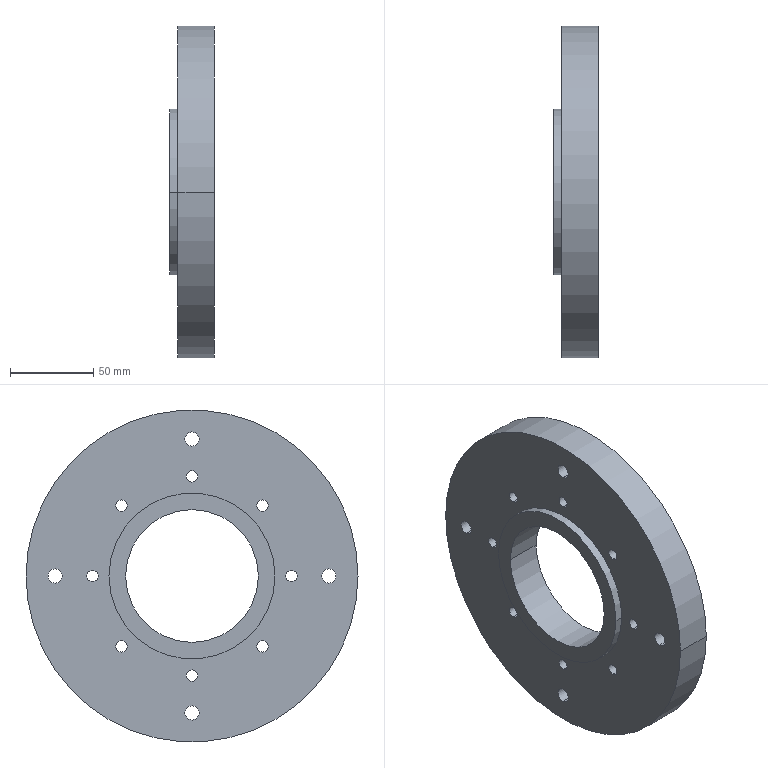Part | STEP file | Motor base plate | 1 solid | 36 faces | box 27 x 200 x 200 mm | volume 543537 mm3 | cylinder 32 | plane 4 | commonest cylinder face diameters 6.8 x16 8.5 x8 80 x2 100 x2 130 x2 200 x2